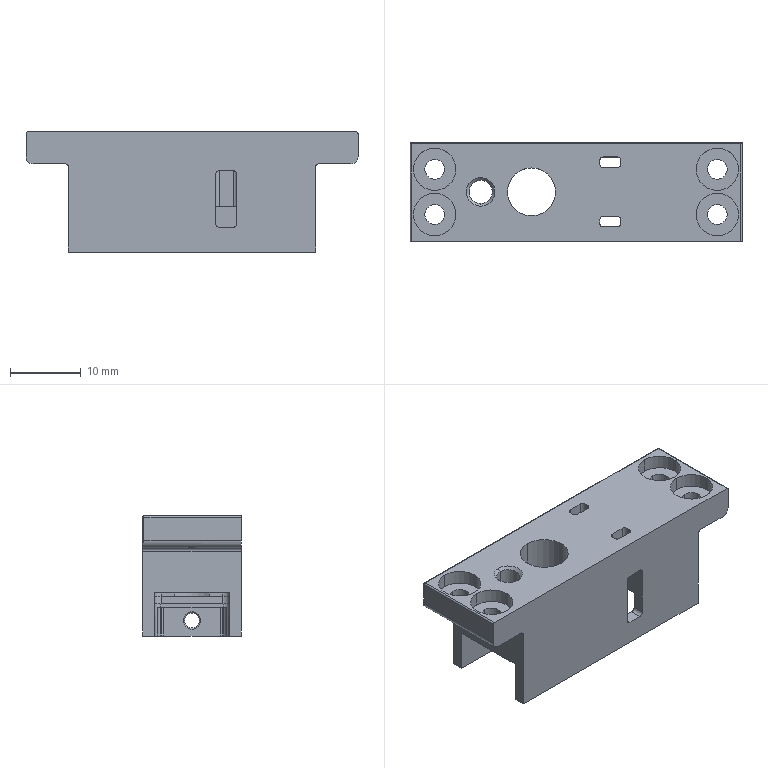NC program | NX | posted with a generic post | part box 47 x 14 x 17 mm
Whole program:
N10 G17 G21 G94 G90
(DRILLING_COPY_1_COPY_1 , TOOL : D6A45)
N12 T18 M6
N14 G54
N16 G17 G0 G90 X0. Y-6.3 B0. C0. S3000 M3
N18 G43 Z30. H18
N20 G94 G81 G98 Z-7.3 F200. R-3.
N22 G80
N24 G0 X0. Y-6.3 Z30.
N26 M5
(DRILLING_COPY_1_COPY_COPY_2 , TOOL : 2.1ZT)
N28 T16 M6
N30 G54
N32 G17 G0 G90 X0. Y-6.3 B0. C0. S2000 M3
N34 G43 Z30. H16
N36 G94 G83 G98 Z-12.416 F150. Q2. R-3.
N38 G80
N40 G0 X0. Y-6.3 Z30.
N42 M5
N44 M2